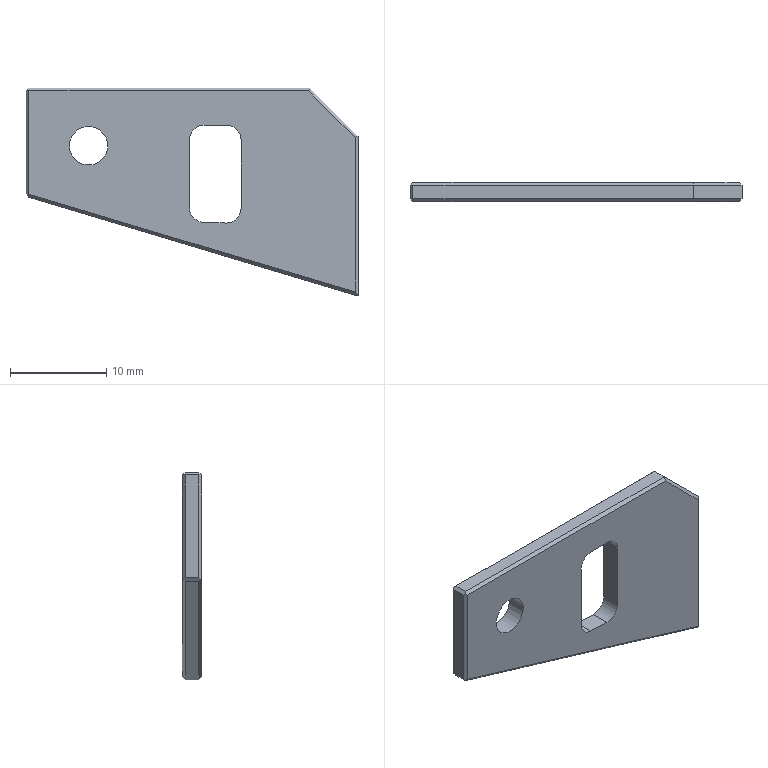Part | NX | 1 solid | 29 faces | box 34.5 x 2 x 21.6 mm | volume 969.552 mm3 | plane 23 | cylinder 6 | commonest cylinder face diameters 3 x4 4 x2
STEP:
#1=CARTESIAN_POINT('',(-158.,156.8,-47.2));
#2=VERTEX_POINT('',#1);
#3=CARTESIAN_POINT('',(-158.,158.2,-47.2));
#4=VERTEX_POINT('',#3);
#5=CARTESIAN_POINT('',(-158.,157.5,-47.2));
#6=DIRECTION('',(0.,1.,0.));
#7=VECTOR('',#6,1000.);
#8=LINE('',#5,#7);
#9=EDGE_CURVE('',#2,#4,#8,.T.);
#10=ORIENTED_EDGE('',*,*,#9,.T.);
#11=CARTESIAN_POINT('',(-158.,158.2,-57.85));
#12=VERTEX_POINT('',#11);
#13=CARTESIAN_POINT('',(-158.,158.2,-52.525));
#14=DIRECTION('',(0.,0.,1.));
#15=VECTOR('',#14,1000.);
#16=LINE('',#13,#15);
#17=EDGE_CURVE('',#12,#4,#16,.T.);
#18=ORIENTED_EDGE('',*,*,#17,.F.);
#19=CARTESIAN_POINT('',(-158.,156.8,-57.85));
#20=VERTEX_POINT('',#19);
#21=CARTESIAN_POINT('',(-158.,157.5,-57.85));
#22=DIRECTION('',(0.,1.,0.));
#23=VECTOR('',#22,1000.);
#24=LINE('',#21,#23);
#25=EDGE_CURVE('',#20,#12,#24,.T.);
#26=ORIENTED_EDGE('',*,*,#25,.F.);
#27=CARTESIAN_POINT('',(-158.,156.8,-52.525));
#28=DIRECTION('',(0.,0.,1.));
#29=VECTOR('',#28,1000.);
#30=LINE('',#27,#29);
#31=EDGE_CURVE('',#20,#2,#30,.T.);
#32=ORIENTED_EDGE('',*,*,#31,.T.);
#33=EDGE_LOOP('',(#10,#18,#26,#32));
#34=FACE_BOUND('',#33,.T.);
#35=CARTESIAN_POINT('',(-158.,156.5,-42.9));
#36=DIRECTION('',(-1.,0.,0.));
#37=DIRECTION('',(0.,0.,1.));
#38=AXIS2_PLACEMENT_3D('',#35,#36,#37);
#39=PLANE('',#38);
#40=ADVANCED_FACE('',(#34),#39,.T.);
#41=CARTESIAN_POINT('',(-128.5,156.8,-46.9));
#42=VERTEX_POINT('',#41);
#43=CARTESIAN_POINT('',(-128.5,158.2,-46.9));
#44=VERTEX_POINT('',#43);
#45=CARTESIAN_POINT('',(-128.5,157.5,-46.9));
#46=DIRECTION('',(0.,1.,0.));
#47=VECTOR('',#46,1000.);
#48=LINE('',#45,#47);
#49=EDGE_CURVE('',#42,#44,#48,.T.);
#50=ORIENTED_EDGE('',*,*,#49,.T.);
#51=CARTESIAN_POINT('',(-157.7,158.2,-46.9));
#52=VERTEX_POINT('',#51);
#53=CARTESIAN_POINT('',(-143.25,158.2,-46.9));
#54=DIRECTION('',(1.,0.,0.));
#55=VECTOR('',#54,1000.);
#56=LINE('',#53,#55);
#57=EDGE_CURVE('',#52,#44,#56,.T.);
#58=ORIENTED_EDGE('',*,*,#57,.F.);
#59=CARTESIAN_POINT('',(-157.7,156.8,-46.9));
#60=VERTEX_POINT('',#59);
#61=CARTESIAN_POINT('',(-157.7,157.5,-46.9));
#62=DIRECTION('',(0.,1.,0.));
#63=VECTOR('',#62,1000.);
#64=LINE('',#61,#63);
#65=EDGE_CURVE('',#60,#52,#64,.T.);
#66=ORIENTED_EDGE('',*,*,#65,.F.);
#67=CARTESIAN_POINT('',(-143.25,156.8,-46.9));
#68=DIRECTION('',(1.,0.,0.));
#69=VECTOR('',#68,1000.);
#70=LINE('',#67,#69);
#71=EDGE_CURVE('',#60,#42,#70,.T.);
#72=ORIENTED_EDGE('',*,*,#71,.T.);
#73=EDGE_LOOP('',(#50,#58,#66,#72));
#74=FACE_BOUND('',#73,.T.);
#75=CARTESIAN_POINT('',(-123.5,156.5,-46.9));
#76=DIRECTION('',(0.,0.,1.));
#77=DIRECTION('',(0.,-1.,0.));
#78=AXIS2_PLACEMENT_3D('',#75,#76,#77);
#79=PLANE('',#78);
#80=ADVANCED_FACE('',(#74),#79,.T.);
#81=CARTESIAN_POINT('',(-123.5,158.2,-51.9));
#82=VERTEX_POINT('',#81);
#83=CARTESIAN_POINT('',(-123.5,158.2,-68.5));
#84=VERTEX_POINT('',#83);
#85=CARTESIAN_POINT('',(-123.5,158.2,-60.2));
#86=DIRECTION('',(0.,0.,-1.));
#87=VECTOR('',#86,1000.);
#88=LINE('',#85,#87);
#89=EDGE_CURVE('',#82,#84,#88,.T.);
#90=ORIENTED_EDGE('',*,*,#89,.F.);
#91=CARTESIAN_POINT('',(-123.5,156.8,-51.9));
#92=VERTEX_POINT('',#91);
#93=CARTESIAN_POINT('',(-123.5,157.5,-51.9));
#94=DIRECTION('',(0.,1.,0.));
#95=VECTOR('',#94,1000.);
#96=LINE('',#93,#95);
#97=EDGE_CURVE('',#92,#82,#96,.T.);
#98=ORIENTED_EDGE('',*,*,#97,.F.);
#99=CARTESIAN_POINT('',(-123.5,156.8,-68.5));
#100=VERTEX_POINT('',#99);
#101=CARTESIAN_POINT('',(-123.5,156.8,-60.2));
#102=DIRECTION('',(0.,0.,-1.));
#103=VECTOR('',#102,1000.);
#104=LINE('',#101,#103);
#105=EDGE_CURVE('',#92,#100,#104,.T.);
#106=ORIENTED_EDGE('',*,*,#105,.T.);
#107=CARTESIAN_POINT('',(-123.5,156.5,-68.5));
#108=DIRECTION('',(0.,-1.,0.));
#109=VECTOR('',#108,1000.);
#110=LINE('',#107,#109);
#111=EDGE_CURVE('',#84,#100,#110,.T.);
#112=ORIENTED_EDGE('',*,*,#111,.F.);
#113=EDGE_LOOP('',(#90,#98,#106,#112));
#114=FACE_BOUND('',#113,.T.);
#115=CARTESIAN_POINT('',(-123.5,156.5,-67.9));
#116=DIRECTION('',(1.,0.,0.));
#117=DIRECTION('',(0.,1.,0.));
#118=AXIS2_PLACEMENT_3D('',#115,#116,#117);
#119=PLANE('',#118);
#120=ADVANCED_FACE('',(#114),#119,.T.);
#121=CARTESIAN_POINT('',(-135.65,156.5,-59.427));
#122=VERTEX_POINT('',#121);
#123=CARTESIAN_POINT('',(-135.65,158.5,-59.427));
#124=VERTEX_POINT('',#123);
#125=CARTESIAN_POINT('',(-135.65,156.5,-59.427));
#126=DIRECTION('',(0.,1.,0.));
#127=VECTOR('',#126,1000.);
#128=LINE('',#125,#127);
#129=EDGE_CURVE('',#122,#124,#128,.T.);
#130=ORIENTED_EDGE('',*,*,#129,.T.);
#131=CARTESIAN_POINT('',(-137.197,158.5,-60.926));
#132=VERTEX_POINT('',#131);
#133=CARTESIAN_POINT('',(-137.15,158.5,-59.427));
#134=DIRECTION('',(0.,1.,0.));
#135=DIRECTION('',(-1.,0.,0.));
#136=AXIS2_PLACEMENT_3D('',#133,#134,#135);
#137=CIRCLE('',#136,1.5);
#138=EDGE_CURVE('',#124,#132,#137,.T.);
#139=ORIENTED_EDGE('',*,*,#138,.T.);
#140=CARTESIAN_POINT('',(-137.197,156.5,-60.926));
#141=VERTEX_POINT('',#140);
#142=CARTESIAN_POINT('',(-137.197,156.5,-60.926));
#143=DIRECTION('',(0.,1.,0.));
#144=VECTOR('',#143,1000.);
#145=LINE('',#142,#144);
#146=EDGE_CURVE('',#141,#132,#145,.T.);
#147=ORIENTED_EDGE('',*,*,#146,.F.);
#148=CARTESIAN_POINT('',(-137.15,156.5,-59.427));
#149=DIRECTION('',(0.,1.,0.));
#150=DIRECTION('',(-1.,0.,0.));
#151=AXIS2_PLACEMENT_3D('',#148,#149,#150);
#152=CIRCLE('',#151,1.5);
#153=EDGE_CURVE('',#122,#141,#152,.T.);
#154=ORIENTED_EDGE('',*,*,#153,.F.);
#155=EDGE_LOOP('',(#130,#139,#147,#154));
#156=FACE_BOUND('',#155,.T.);
#157=CARTESIAN_POINT('',(-137.15,156.5,-59.427));
#158=DIRECTION('',(0.,1.,0.));
#159=DIRECTION('',(-1.,0.,0.));
#160=AXIS2_PLACEMENT_3D('',#157,#158,#159);
#161=CYLINDRICAL_SURFACE('',#160,1.5);
#162=ADVANCED_FACE('',(#156),#161,.F.);
#163=ORIENTED_EDGE('',*,*,#111,.T.);
#164=CARTESIAN_POINT('',(-157.713,156.8,-58.236));
#165=VERTEX_POINT('',#164);
#166=CARTESIAN_POINT('',(-140.75,156.8,-63.325));
#167=DIRECTION('',(-0.9578,0.,0.2873));
#168=VECTOR('',#167,1000.);
#169=LINE('',#166,#168);
#170=EDGE_CURVE('',#100,#165,#169,.T.);
#171=ORIENTED_EDGE('',*,*,#170,.T.);
#172=CARTESIAN_POINT('',(-157.713,158.2,-58.236));
#173=VERTEX_POINT('',#172);
#174=CARTESIAN_POINT('',(-157.713,157.5,-58.236));
#175=DIRECTION('',(0.,1.,0.));
#176=VECTOR('',#175,1000.);
#177=LINE('',#174,#176);
#178=EDGE_CURVE('',#165,#173,#177,.T.);
#179=ORIENTED_EDGE('',*,*,#178,.T.);
#180=CARTESIAN_POINT('',(-140.75,158.2,-63.325));
#181=DIRECTION('',(-0.9578,0.,0.2873));
#182=VECTOR('',#181,1000.);
#183=LINE('',#180,#182);
#184=EDGE_CURVE('',#84,#173,#183,.T.);
#185=ORIENTED_EDGE('',*,*,#184,.F.);
#186=EDGE_LOOP('',(#163,#171,#179,#185));
#187=FACE_BOUND('',#186,.T.);
#188=CARTESIAN_POINT('',(-160.5,156.5,-57.4));
#189=DIRECTION('',(-0.2873,0.,-0.9578));
#190=DIRECTION('',(-0.9578,0.,0.2873));
#191=AXIS2_PLACEMENT_3D('',#188,#189,#190);
#192=PLANE('',#191);
#193=ADVANCED_FACE('',(#187),#192,.T.);
#194=CARTESIAN_POINT('',(-141.001,156.5,-59.354));
#195=VERTEX_POINT('',#194);
#196=CARTESIAN_POINT('',(-141.001,158.5,-59.354));
#197=VERTEX_POINT('',#196);
#198=CARTESIAN_POINT('',(-141.001,156.5,-59.354));
#199=DIRECTION('',(0.,1.,0.));
#200=VECTOR('',#199,1000.);
#201=LINE('',#198,#200);
#202=EDGE_CURVE('',#195,#197,#201,.T.);
#203=ORIENTED_EDGE('',*,*,#202,.F.);
#204=CARTESIAN_POINT('',(-139.548,156.5,-60.853));
#205=VERTEX_POINT('',#204);
#206=CARTESIAN_POINT('',(-139.501,156.5,-59.354));
#207=DIRECTION('',(0.,1.,0.));
#208=DIRECTION('',(-1.,0.,0.));
#209=AXIS2_PLACEMENT_3D('',#206,#207,#208);
#210=CIRCLE('',#209,1.5);
#211=EDGE_CURVE('',#205,#195,#210,.T.);
#212=ORIENTED_EDGE('',*,*,#211,.F.);
#213=CARTESIAN_POINT('',(-139.548,158.5,-60.853));
#214=VERTEX_POINT('',#213);
#215=CARTESIAN_POINT('',(-139.548,156.5,-60.853));
#216=DIRECTION('',(0.,1.,0.));
#217=VECTOR('',#216,1000.);
#218=LINE('',#215,#217);
#219=EDGE_CURVE('',#205,#214,#218,.T.);
#220=ORIENTED_EDGE('',*,*,#219,.T.);
#221=CARTESIAN_POINT('',(-139.501,158.5,-59.354));
#222=DIRECTION('',(0.,1.,0.));
#223=DIRECTION('',(-1.,0.,0.));
#224=AXIS2_PLACEMENT_3D('',#221,#222,#223);
#225=CIRCLE('',#224,1.5);
#226=EDGE_CURVE('',#214,#197,#225,.T.);
#227=ORIENTED_EDGE('',*,*,#226,.T.);
#228=EDGE_LOOP('',(#203,#212,#220,#227));
#229=FACE_BOUND('',#228,.T.);
#230=CARTESIAN_POINT('',(-139.501,156.5,-59.354));
#231=DIRECTION('',(0.,1.,0.));
#232=DIRECTION('',(-1.,0.,0.));
#233=AXIS2_PLACEMENT_3D('',#230,#231,#232);
#234=CYLINDRICAL_SURFACE('',#233,1.5);
#235=ADVANCED_FACE('',(#229),#234,.F.);
#236=CARTESIAN_POINT('',(-137.15,156.5,-50.763));
#237=VERTEX_POINT('',#236);
#238=CARTESIAN_POINT('',(-137.15,158.5,-50.763));
#239=VERTEX_POINT('',#238);
#240=CARTESIAN_POINT('',(-137.15,156.5,-50.763));
#241=DIRECTION('',(0.,1.,0.));
#242=VECTOR('',#241,1000.);
#243=LINE('',#240,#242);
#244=EDGE_CURVE('',#237,#239,#243,.T.);
#245=ORIENTED_EDGE('',*,*,#244,.F.);
#246=CARTESIAN_POINT('',(-139.501,156.5,-50.763));
#247=VERTEX_POINT('',#246);
#248=CARTESIAN_POINT('',(-108.092,156.5,-50.763));
#249=DIRECTION('',(1.,0.,0.));
#250=VECTOR('',#249,1000.);
#251=LINE('',#248,#250);
#252=EDGE_CURVE('',#247,#237,#251,.T.);
#253=ORIENTED_EDGE('',*,*,#252,.F.);
#254=CARTESIAN_POINT('',(-139.501,158.5,-50.763));
#255=VERTEX_POINT('',#254);
#256=CARTESIAN_POINT('',(-139.501,156.5,-50.763));
#257=DIRECTION('',(0.,1.,0.));
#258=VECTOR('',#257,1000.);
#259=LINE('',#256,#258);
#260=EDGE_CURVE('',#247,#255,#259,.T.);
#261=ORIENTED_EDGE('',*,*,#260,.T.);
#262=CARTESIAN_POINT('',(-108.092,158.5,-50.763));
#263=DIRECTION('',(1.,0.,0.));
#264=VECTOR('',#263,1000.);
#265=LINE('',#262,#264);
#266=EDGE_CURVE('',#255,#239,#265,.T.);
#267=ORIENTED_EDGE('',*,*,#266,.T.);
#268=EDGE_LOOP('',(#245,#253,#261,#267));
#269=FACE_BOUND('',#268,.T.);
#270=CARTESIAN_POINT('',(-135.65,156.3,-50.763));
#271=DIRECTION('',(0.,0.,1.));
#272=DIRECTION('',(0.,-1.,0.));
#273=AXIS2_PLACEMENT_3D('',#270,#271,#272);
#274=PLANE('',#273);
#275=ADVANCED_FACE('',(#269),#274,.F.);
#276=ORIENTED_EDGE('',*,*,#129,.F.);
#277=CARTESIAN_POINT('',(-135.65,156.5,-52.263));
#278=VERTEX_POINT('',#277);
#279=CARTESIAN_POINT('',(-135.65,156.5,-58.685));
#280=DIRECTION('',(0.,0.,-1.));
#281=VECTOR('',#280,1000.);
#282=LINE('',#279,#281);
#283=EDGE_CURVE('',#278,#122,#282,.T.);
#284=ORIENTED_EDGE('',*,*,#283,.F.);
#285=CARTESIAN_POINT('',(-135.65,158.5,-52.263));
#286=VERTEX_POINT('',#285);
#287=CARTESIAN_POINT('',(-135.65,156.5,-52.263));
#288=DIRECTION('',(0.,1.,0.));
#289=VECTOR('',#288,1000.);
#290=LINE('',#287,#289);
#291=EDGE_CURVE('',#278,#286,#290,.T.);
#292=ORIENTED_EDGE('',*,*,#291,.T.);
#293=CARTESIAN_POINT('',(-135.65,158.5,-58.685));
#294=DIRECTION('',(0.,0.,-1.));
#295=VECTOR('',#294,1000.);
#296=LINE('',#293,#295);
#297=EDGE_CURVE('',#286,#124,#296,.T.);
#298=ORIENTED_EDGE('',*,*,#297,.T.);
#299=EDGE_LOOP('',(#276,#284,#292,#298));
#300=FACE_BOUND('',#299,.T.);
#301=CARTESIAN_POINT('',(-135.65,156.3,-60.975));
#302=DIRECTION('',(1.,0.,0.));
#303=DIRECTION('',(0.,0.,-1.));
#304=AXIS2_PLACEMENT_3D('',#301,#302,#303);
#305=PLANE('',#304);
#306=ADVANCED_FACE('',(#300),#305,.F.);
#307=CARTESIAN_POINT('',(-108.092,158.5,-61.836));
#308=DIRECTION('',(-0.9995,0.,0.03124));
#309=VECTOR('',#308,1000.);
#310=LINE('',#307,#309);
#311=EDGE_CURVE('',#132,#214,#310,.T.);
#312=ORIENTED_EDGE('',*,*,#311,.T.);
#313=ORIENTED_EDGE('',*,*,#219,.F.);
#314=CARTESIAN_POINT('',(-108.092,156.5,-61.836));
#315=DIRECTION('',(-0.9995,0.,0.03124));
#316=VECTOR('',#315,1000.);
#317=LINE('',#314,#316);
#318=EDGE_CURVE('',#141,#205,#317,.T.);
#319=ORIENTED_EDGE('',*,*,#318,.F.);
#320=ORIENTED_EDGE('',*,*,#146,.T.);
#321=EDGE_LOOP('',(#312,#313,#319,#320));
#322=FACE_BOUND('',#321,.T.);
#323=CARTESIAN_POINT('',(-141.001,156.3,-60.807));
#324=DIRECTION('',(-0.03124,0.,-0.9995));
#325=DIRECTION('',(-0.9995,0.,0.03124));
#326=AXIS2_PLACEMENT_3D('',#323,#324,#325);
#327=PLANE('',#326);
#328=ADVANCED_FACE('',(#322),#327,.F.);
#329=ORIENTED_EDGE('',*,*,#202,.T.);
#330=CARTESIAN_POINT('',(-141.001,158.5,-52.263));
#331=VERTEX_POINT('',#330);
#332=CARTESIAN_POINT('',(-141.001,158.5,-58.685));
#333=DIRECTION('',(0.,0.,1.));
#334=VECTOR('',#333,1000.);
#335=LINE('',#332,#334);
#336=EDGE_CURVE('',#197,#331,#335,.T.);
#337=ORIENTED_EDGE('',*,*,#336,.T.);
#338=CARTESIAN_POINT('',(-141.001,156.5,-52.263));
#339=VERTEX_POINT('',#338);
#340=CARTESIAN_POINT('',(-141.001,156.5,-52.263));
#341=DIRECTION('',(0.,1.,0.));
#342=VECTOR('',#341,1000.);
#343=LINE('',#340,#342);
#344=EDGE_CURVE('',#339,#331,#343,.T.);
#345=ORIENTED_EDGE('',*,*,#344,.F.);
#346=CARTESIAN_POINT('',(-141.001,156.5,-58.685));
#347=DIRECTION('',(0.,0.,1.));
#348=VECTOR('',#347,1000.);
#349=LINE('',#346,#348);
#350=EDGE_CURVE('',#195,#339,#349,.T.);
#351=ORIENTED_EDGE('',*,*,#350,.F.);
#352=EDGE_LOOP('',(#329,#337,#345,#351));
#353=FACE_BOUND('',#352,.T.);
#354=CARTESIAN_POINT('',(-141.001,156.3,-50.763));
#355=DIRECTION('',(-1.,0.,0.));
#356=DIRECTION('',(0.,0.,1.));
#357=AXIS2_PLACEMENT_3D('',#354,#355,#356);
#358=PLANE('',#357);
#359=ADVANCED_FACE('',(#353),#358,.F.);
#360=ORIENTED_EDGE('',*,*,#344,.T.);
#361=CARTESIAN_POINT('',(-139.501,158.5,-52.263));
#362=DIRECTION('',(0.,1.,0.));
#363=DIRECTION('',(-1.,0.,0.));
#364=AXIS2_PLACEMENT_3D('',#361,#362,#363);
#365=CIRCLE('',#364,1.5);
#366=EDGE_CURVE('',#331,#255,#365,.T.);
#367=ORIENTED_EDGE('',*,*,#366,.T.);
#368=ORIENTED_EDGE('',*,*,#260,.F.);
#369=CARTESIAN_POINT('',(-139.501,156.5,-52.263));
#370=DIRECTION('',(0.,1.,0.));
#371=DIRECTION('',(-1.,0.,0.));
#372=AXIS2_PLACEMENT_3D('',#369,#370,#371);
#373=CIRCLE('',#372,1.5);
#374=EDGE_CURVE('',#339,#247,#373,.T.);
#375=ORIENTED_EDGE('',*,*,#374,.F.);
#376=EDGE_LOOP('',(#360,#367,#368,#375));
#377=FACE_BOUND('',#376,.T.);
#378=CARTESIAN_POINT('',(-139.501,156.5,-52.263));
#379=DIRECTION('',(0.,1.,0.));
#380=DIRECTION('',(-1.,0.,0.));
#381=AXIS2_PLACEMENT_3D('',#378,#379,#380);
#382=CYLINDRICAL_SURFACE('',#381,1.5);
#383=ADVANCED_FACE('',(#377),#382,.F.);
#384=ORIENTED_EDGE('',*,*,#244,.T.);
#385=CARTESIAN_POINT('',(-137.15,158.5,-52.263));
#386=DIRECTION('',(0.,1.,0.));
#387=DIRECTION('',(-1.,0.,0.));
#388=AXIS2_PLACEMENT_3D('',#385,#386,#387);
#389=CIRCLE('',#388,1.5);
#390=EDGE_CURVE('',#239,#286,#389,.T.);
#391=ORIENTED_EDGE('',*,*,#390,.T.);
#392=ORIENTED_EDGE('',*,*,#291,.F.);
#393=CARTESIAN_POINT('',(-137.15,156.5,-52.263));
#394=DIRECTION('',(0.,1.,0.));
#395=DIRECTION('',(-1.,0.,0.));
#396=AXIS2_PLACEMENT_3D('',#393,#394,#395);
#397=CIRCLE('',#396,1.5);
#398=EDGE_CURVE('',#237,#278,#397,.T.);
#399=ORIENTED_EDGE('',*,*,#398,.F.);
#400=EDGE_LOOP('',(#384,#391,#392,#399));
#401=FACE_BOUND('',#400,.T.);
#402=CARTESIAN_POINT('',(-137.15,156.5,-52.263));
#403=DIRECTION('',(0.,1.,0.));
#404=DIRECTION('',(-1.,0.,0.));
#405=AXIS2_PLACEMENT_3D('',#402,#403,#404);
#406=CYLINDRICAL_SURFACE('',#405,1.5);
#407=ADVANCED_FACE('',(#401),#406,.F.);
#408=CARTESIAN_POINT('',(-126.,158.2,-49.4));
#409=DIRECTION('',(-0.7071,0.,0.7071));
#410=VECTOR('',#409,1000.);
#411=LINE('',#408,#410);
#412=EDGE_CURVE('',#82,#44,#411,.T.);
#413=ORIENTED_EDGE('',*,*,#412,.T.);
#414=ORIENTED_EDGE('',*,*,#49,.F.);
#415=CARTESIAN_POINT('',(-126.,156.8,-49.4));
#416=DIRECTION('',(-0.7071,0.,0.7071));
#417=VECTOR('',#416,1000.);
#418=LINE('',#415,#417);
#419=EDGE_CURVE('',#92,#42,#418,.T.);
#420=ORIENTED_EDGE('',*,*,#419,.F.);
#421=ORIENTED_EDGE('',*,*,#97,.T.);
#422=EDGE_LOOP('',(#413,#414,#420,#421));
#423=FACE_BOUND('',#422,.T.);
#424=CARTESIAN_POINT('',(-126.,157.5,-49.4));
#425=DIRECTION('',(0.7071,0.,0.7071));
#426=DIRECTION('',(0.,-1.,0.));
#427=AXIS2_PLACEMENT_3D('',#424,#425,#426);
#428=PLANE('',#427);
#429=ADVANCED_FACE('',(#423),#428,.T.);
#430=ORIENTED_EDGE('',*,*,#25,.T.);
#431=CARTESIAN_POINT('',(-157.856,158.344,-58.043));
#432=VERTEX_POINT('',#431);
#433=CARTESIAN_POINT('',(-157.379,158.821,-58.685));
#434=DIRECTION('',(0.5126,0.5126,-0.6889));
#435=VECTOR('',#434,1000.);
#436=LINE('',#433,#435);
#437=EDGE_CURVE('',#12,#432,#436,.T.);
#438=ORIENTED_EDGE('',*,*,#437,.T.);
#439=CARTESIAN_POINT('',(-157.379,157.866,-58.685));
#440=DIRECTION('',(0.5126,-0.5126,-0.6889));
#441=VECTOR('',#440,1000.);
#442=LINE('',#439,#441);
#443=EDGE_CURVE('',#432,#173,#442,.T.);
#444=ORIENTED_EDGE('',*,*,#443,.T.);
#445=ORIENTED_EDGE('',*,*,#178,.F.);
#446=CARTESIAN_POINT('',(-157.856,156.656,-58.043));
#447=VERTEX_POINT('',#446);
#448=CARTESIAN_POINT('',(-157.379,157.134,-58.685));
#449=DIRECTION('',(0.5126,0.5126,-0.6889));
#450=VECTOR('',#449,1000.);
#451=LINE('',#448,#450);
#452=EDGE_CURVE('',#447,#165,#451,.T.);
#453=ORIENTED_EDGE('',*,*,#452,.F.);
#454=CARTESIAN_POINT('',(-157.379,156.179,-58.685));
#455=DIRECTION('',(0.5126,-0.5126,-0.6889));
#456=VECTOR('',#455,1000.);
#457=LINE('',#454,#456);
#458=EDGE_CURVE('',#20,#447,#457,.T.);
#459=ORIENTED_EDGE('',*,*,#458,.F.);
#460=EDGE_LOOP('',(#430,#438,#444,#445,#453,#459));
#461=FACE_BOUND('',#460,.T.);
#462=CARTESIAN_POINT('',(-157.856,157.5,-58.043));
#463=DIRECTION('',(0.8023,0.,0.5969));
#464=DIRECTION('',(0.,-1.,0.));
#465=AXIS2_PLACEMENT_3D('',#462,#463,#464);
#466=PLANE('',#465);
#467=ADVANCED_FACE('',(#461),#466,.F.);
#468=ORIENTED_EDGE('',*,*,#9,.F.);
#469=CARTESIAN_POINT('',(-157.85,156.65,-47.05));
#470=VERTEX_POINT('',#469);
#471=CARTESIAN_POINT('',(-169.485,168.285,-58.685));
#472=DIRECTION('',(0.5774,-0.5774,0.5774));
#473=VECTOR('',#472,1000.);
#474=LINE('',#471,#473);
#475=EDGE_CURVE('',#2,#470,#474,.T.);
#476=ORIENTED_EDGE('',*,*,#475,.T.);
#477=CARTESIAN_POINT('',(-169.485,145.015,-58.685));
#478=DIRECTION('',(0.5774,0.5774,0.5774));
#479=VECTOR('',#478,1000.);
#480=LINE('',#477,#479);
#481=EDGE_CURVE('',#470,#60,#480,.T.);
#482=ORIENTED_EDGE('',*,*,#481,.T.);
#483=ORIENTED_EDGE('',*,*,#65,.T.);
#484=CARTESIAN_POINT('',(-157.85,158.35,-47.05));
#485=VERTEX_POINT('',#484);
#486=CARTESIAN_POINT('',(-169.485,169.985,-58.685));
#487=DIRECTION('',(0.5774,-0.5774,0.5774));
#488=VECTOR('',#487,1000.);
#489=LINE('',#486,#488);
#490=EDGE_CURVE('',#485,#52,#489,.T.);
#491=ORIENTED_EDGE('',*,*,#490,.F.);
#492=CARTESIAN_POINT('',(-169.485,146.715,-58.685));
#493=DIRECTION('',(0.5774,0.5774,0.5774));
#494=VECTOR('',#493,1000.);
#495=LINE('',#492,#494);
#496=EDGE_CURVE('',#4,#485,#495,.T.);
#497=ORIENTED_EDGE('',*,*,#496,.F.);
#498=EDGE_LOOP('',(#468,#476,#482,#483,#491,#497));
#499=FACE_BOUND('',#498,.T.);
#500=CARTESIAN_POINT('',(-157.85,157.5,-47.05));
#501=DIRECTION('',(-0.7071,0.,0.7071));
#502=DIRECTION('',(0.,1.,0.));
#503=AXIS2_PLACEMENT_3D('',#500,#501,#502);
#504=PLANE('',#503);
#505=ADVANCED_FACE('',(#499),#504,.T.);
#506=ORIENTED_EDGE('',*,*,#419,.T.);
#507=CARTESIAN_POINT('',(-128.624,156.5,-47.2));
#508=VERTEX_POINT('',#507);
#509=CARTESIAN_POINT('',(-133.381,145.015,-58.685));
#510=DIRECTION('',(0.2811,0.6786,0.6786));
#511=VECTOR('',#510,1000.);
#512=LINE('',#509,#511);
#513=EDGE_CURVE('',#508,#42,#512,.T.);
#514=ORIENTED_EDGE('',*,*,#513,.F.);
#515=CARTESIAN_POINT('',(-123.8,156.5,-52.024));
#516=VERTEX_POINT('',#515);
#517=CARTESIAN_POINT('',(-126.212,156.5,-49.612));
#518=DIRECTION('',(-0.7071,0.,0.7071));
#519=VECTOR('',#518,1000.);
#520=LINE('',#517,#519);
#521=EDGE_CURVE('',#516,#508,#520,.T.);
#522=ORIENTED_EDGE('',*,*,#521,.F.);
#523=CARTESIAN_POINT('',(-108.092,172.208,-45.518));
#524=DIRECTION('',(-0.6786,-0.6786,-0.2811));
#525=VECTOR('',#524,1000.);
#526=LINE('',#523,#525);
#527=EDGE_CURVE('',#92,#516,#526,.T.);
#528=ORIENTED_EDGE('',*,*,#527,.F.);
#529=EDGE_LOOP('',(#506,#514,#522,#528));
#530=FACE_BOUND('',#529,.T.);
#531=CARTESIAN_POINT('',(-126.106,156.65,-49.506));
#532=DIRECTION('',(-0.5,0.7071,-0.5));
#533=DIRECTION('',(-0.7071,0.,0.7071));
#534=AXIS2_PLACEMENT_3D('',#531,#532,#533);
#535=PLANE('',#534);
#536=ADVANCED_FACE('',(#530),#535,.F.);
#537=ORIENTED_EDGE('',*,*,#412,.F.);
#538=CARTESIAN_POINT('',(-123.8,158.5,-52.024));
#539=VERTEX_POINT('',#538);
#540=CARTESIAN_POINT('',(-108.092,142.792,-45.518));
#541=DIRECTION('',(0.6786,-0.6786,0.2811));
#542=VECTOR('',#541,1000.);
#543=LINE('',#540,#542);
#544=EDGE_CURVE('',#539,#82,#543,.T.);
#545=ORIENTED_EDGE('',*,*,#544,.F.);
#546=CARTESIAN_POINT('',(-128.624,158.5,-47.2));
#547=VERTEX_POINT('',#546);
#548=CARTESIAN_POINT('',(-126.212,158.5,-49.612));
#549=DIRECTION('',(-0.7071,0.,0.7071));
#550=VECTOR('',#549,1000.);
#551=LINE('',#548,#550);
#552=EDGE_CURVE('',#539,#547,#551,.T.);
#553=ORIENTED_EDGE('',*,*,#552,.T.);
#554=CARTESIAN_POINT('',(-133.381,169.985,-58.685));
#555=DIRECTION('',(-0.2811,0.6786,-0.6786));
#556=VECTOR('',#555,1000.);
#557=LINE('',#554,#556);
#558=EDGE_CURVE('',#44,#547,#557,.T.);
#559=ORIENTED_EDGE('',*,*,#558,.F.);
#560=EDGE_LOOP('',(#537,#545,#553,#559));
#561=FACE_BOUND('',#560,.T.);
#562=CARTESIAN_POINT('',(-126.106,158.35,-49.506));
#563=DIRECTION('',(0.5,0.7071,0.5));
#564=DIRECTION('',(0.7071,0.,-0.7071));
#565=AXIS2_PLACEMENT_3D('',#562,#563,#564);
#566=PLANE('',#565);
#567=ADVANCED_FACE('',(#561),#566,.T.);
#568=CARTESIAN_POINT('',(-149.5,158.5,-52.9));
#569=VERTEX_POINT('',#568);
#570=CARTESIAN_POINT('',(-153.5,158.5,-52.9));
#571=VERTEX_POINT('',#570);
#572=CARTESIAN_POINT('',(-151.5,158.5,-52.9));
#573=DIRECTION('',(0.,1.,0.));
#574=DIRECTION('',(-1.,0.,0.));
#575=AXIS2_PLACEMENT_3D('',#572,#573,#574);
#576=CIRCLE('',#575,2.);
#577=EDGE_CURVE('',#569,#571,#576,.T.);
#578=ORIENTED_EDGE('',*,*,#577,.T.);
#579=CARTESIAN_POINT('',(-153.5,156.5,-52.9));
#580=VERTEX_POINT('',#579);
#581=CARTESIAN_POINT('',(-153.5,156.5,-52.9));
#582=DIRECTION('',(0.,1.,0.));
#583=VECTOR('',#582,1000.);
#584=LINE('',#581,#583);
#585=EDGE_CURVE('',#571,#580,#584,.F.);
#586=ORIENTED_EDGE('',*,*,#585,.T.);
#587=CARTESIAN_POINT('',(-149.5,156.5,-52.9));
#588=VERTEX_POINT('',#587);
#589=CARTESIAN_POINT('',(-151.5,156.5,-52.9));
#590=DIRECTION('',(0.,1.,0.));
#591=DIRECTION('',(-1.,0.,0.));
#592=AXIS2_PLACEMENT_3D('',#589,#590,#591);
#593=CIRCLE('',#592,2.);
#594=EDGE_CURVE('',#588,#580,#593,.T.);
#595=ORIENTED_EDGE('',*,*,#594,.F.);
#596=CARTESIAN_POINT('',(-149.5,156.5,-52.9));
#597=DIRECTION('',(0.,1.,0.));
#598=VECTOR('',#597,1000.);
#599=LINE('',#596,#598);
#600=EDGE_CURVE('',#569,#588,#599,.F.);
#601=ORIENTED_EDGE('',*,*,#600,.F.);
#602=EDGE_LOOP('',(#578,#586,#595,#601));
#603=FACE_BOUND('',#602,.T.);
#604=CARTESIAN_POINT('',(-151.5,156.5,-52.9));
#605=DIRECTION('',(0.,1.,0.));
#606=DIRECTION('',(-1.,0.,0.));
#607=AXIS2_PLACEMENT_3D('',#604,#605,#606);
#608=CYLINDRICAL_SURFACE('',#607,2.);
#609=ADVANCED_FACE('',(#603),#608,.F.);
#610=ORIENTED_EDGE('',*,*,#585,.F.);
#611=CARTESIAN_POINT('',(-151.5,158.5,-52.9));
#612=DIRECTION('',(0.,1.,0.));
#613=DIRECTION('',(-1.,0.,0.));
#614=AXIS2_PLACEMENT_3D('',#611,#612,#613);
#615=CIRCLE('',#614,2.);
#616=EDGE_CURVE('',#571,#569,#615,.T.);
#617=ORIENTED_EDGE('',*,*,#616,.T.);
#618=ORIENTED_EDGE('',*,*,#600,.T.);
#619=CARTESIAN_POINT('',(-151.5,156.5,-52.9));
#620=DIRECTION('',(0.,1.,0.));
#621=DIRECTION('',(-1.,0.,0.));
#622=AXIS2_PLACEMENT_3D('',#619,#620,#621);
#623=CIRCLE('',#622,2.);
#624=EDGE_CURVE('',#580,#588,#623,.T.);
#625=ORIENTED_EDGE('',*,*,#624,.F.);
#626=EDGE_LOOP('',(#610,#617,#618,#625));
#627=FACE_BOUND('',#626,.T.);
#628=CARTESIAN_POINT('',(-151.5,156.5,-52.9));
#629=DIRECTION('',(0.,1.,0.));
#630=DIRECTION('',(-1.,0.,0.));
#631=AXIS2_PLACEMENT_3D('',#628,#629,#630);
#632=CYLINDRICAL_SURFACE('',#631,2.);
#633=ADVANCED_FACE('',(#627),#632,.F.);
#634=CARTESIAN_POINT('',(-157.7,158.5,-57.927));
#635=VERTEX_POINT('',#634);
#636=CARTESIAN_POINT('',(-157.7,158.5,-47.2));
#637=VERTEX_POINT('',#636);
#638=CARTESIAN_POINT('',(-157.7,158.5,-52.525));
#639=DIRECTION('',(0.,0.,1.));
#640=VECTOR('',#639,1000.);
#641=LINE('',#638,#640);
#642=EDGE_CURVE('',#635,#637,#641,.T.);
#643=ORIENTED_EDGE('',*,*,#642,.T.);
#644=CARTESIAN_POINT('',(-143.25,158.5,-47.2));
#645=DIRECTION('',(1.,0.,0.));
#646=VECTOR('',#645,1000.);
#647=LINE('',#644,#646);
#648=EDGE_CURVE('',#637,#547,#647,.T.);
#649=ORIENTED_EDGE('',*,*,#648,.T.);
#650=ORIENTED_EDGE('',*,*,#552,.F.);
#651=CARTESIAN_POINT('',(-123.8,158.5,-68.097));
#652=VERTEX_POINT('',#651);
#653=CARTESIAN_POINT('',(-123.8,158.5,-60.2));
#654=DIRECTION('',(0.,0.,-1.));
#655=VECTOR('',#654,1000.);
#656=LINE('',#653,#655);
#657=EDGE_CURVE('',#539,#652,#656,.T.);
#658=ORIENTED_EDGE('',*,*,#657,.T.);
#659=CARTESIAN_POINT('',(-140.664,158.5,-63.038));
#660=DIRECTION('',(-0.9578,0.,0.2873));
#661=VECTOR('',#660,1000.);
#662=LINE('',#659,#661);
#663=EDGE_CURVE('',#652,#635,#662,.T.);
#664=ORIENTED_EDGE('',*,*,#663,.T.);
#665=EDGE_LOOP('',(#643,#649,#650,#658,#664));
#666=FACE_BOUND('',#665,.T.);
#667=ORIENTED_EDGE('',*,*,#336,.F.);
#668=ORIENTED_EDGE('',*,*,#226,.F.);
#669=ORIENTED_EDGE('',*,*,#311,.F.);
#670=ORIENTED_EDGE('',*,*,#138,.F.);
#671=ORIENTED_EDGE('',*,*,#297,.F.);
#672=ORIENTED_EDGE('',*,*,#390,.F.);
#673=ORIENTED_EDGE('',*,*,#266,.F.);
#674=ORIENTED_EDGE('',*,*,#366,.F.);
#675=EDGE_LOOP('',(#667,#668,#669,#670,#671,#672,#673,#674));
#676=FACE_BOUND('',#675,.T.);
#677=ORIENTED_EDGE('',*,*,#577,.F.);
#678=ORIENTED_EDGE('',*,*,#616,.F.);
#679=EDGE_LOOP('',(#677,#678));
#680=FACE_BOUND('',#679,.T.);
#681=CARTESIAN_POINT('',(-108.092,158.5,-58.685));
#682=DIRECTION('',(0.,1.,0.));
#683=DIRECTION('',(0.,0.,-1.));
#684=AXIS2_PLACEMENT_3D('',#681,#682,#683);
#685=PLANE('',#684);
#686=ADVANCED_FACE('',(#666,#676,#680),#685,.T.);
#687=ORIENTED_EDGE('',*,*,#657,.F.);
#688=ORIENTED_EDGE('',*,*,#544,.T.);
#689=ORIENTED_EDGE('',*,*,#89,.T.);
#690=CARTESIAN_POINT('',(-130.803,165.503,-58.685));
#691=DIRECTION('',(-0.5126,0.5126,0.6889));
#692=VECTOR('',#691,1000.);
#693=LINE('',#690,#692);
#694=EDGE_CURVE('',#84,#652,#693,.T.);
#695=ORIENTED_EDGE('',*,*,#694,.T.);
#696=EDGE_LOOP('',(#687,#688,#689,#695));
#697=FACE_BOUND('',#696,.T.);
#698=CARTESIAN_POINT('',(-123.65,158.35,-60.2));
#699=DIRECTION('',(0.7071,0.7071,0.));
#700=DIRECTION('',(0.,0.,-1.));
#701=AXIS2_PLACEMENT_3D('',#698,#699,#700);
#702=PLANE('',#701);
#703=ADVANCED_FACE('',(#697),#702,.T.);
#704=ORIENTED_EDGE('',*,*,#648,.F.);
#705=CARTESIAN_POINT('',(-146.215,169.985,-58.685));
#706=DIRECTION('',(-0.5774,-0.5774,0.5774));
#707=VECTOR('',#706,1000.);
#708=LINE('',#705,#707);
#709=EDGE_CURVE('',#637,#485,#708,.T.);
#710=ORIENTED_EDGE('',*,*,#709,.T.);
#711=ORIENTED_EDGE('',*,*,#490,.T.);
#712=ORIENTED_EDGE('',*,*,#57,.T.);
#713=ORIENTED_EDGE('',*,*,#558,.T.);
#714=EDGE_LOOP('',(#704,#710,#711,#712,#713));
#715=FACE_BOUND('',#714,.T.);
#716=CARTESIAN_POINT('',(-143.25,158.35,-47.05));
#717=DIRECTION('',(0.,0.7071,0.7071));
#718=DIRECTION('',(1.,0.,0.));
#719=AXIS2_PLACEMENT_3D('',#716,#717,#718);
#720=PLANE('',#719);
#721=ADVANCED_FACE('',(#715),#720,.T.);
#722=ORIENTED_EDGE('',*,*,#663,.F.);
#723=ORIENTED_EDGE('',*,*,#694,.F.);
#724=ORIENTED_EDGE('',*,*,#184,.T.);
#725=ORIENTED_EDGE('',*,*,#443,.F.);
#726=CARTESIAN_POINT('',(-159.7,156.5,-59.415));
#727=DIRECTION('',(0.6258,0.6258,0.4656));
#728=VECTOR('',#727,1000.);
#729=LINE('',#726,#728);
#730=EDGE_CURVE('',#432,#635,#729,.T.);
#731=ORIENTED_EDGE('',*,*,#730,.T.);
#732=EDGE_LOOP('',(#722,#723,#724,#725,#731));
#733=FACE_BOUND('',#732,.T.);
#734=CARTESIAN_POINT('',(-140.707,158.35,-63.181));
#735=DIRECTION('',(-0.2032,0.7071,-0.6773));
#736=DIRECTION('',(-0.9578,0.,0.2873));
#737=AXIS2_PLACEMENT_3D('',#734,#735,#736);
#738=PLANE('',#737);
#739=ADVANCED_FACE('',(#733),#738,.T.);
#740=ORIENTED_EDGE('',*,*,#642,.F.);
#741=ORIENTED_EDGE('',*,*,#730,.F.);
#742=ORIENTED_EDGE('',*,*,#437,.F.);
#743=ORIENTED_EDGE('',*,*,#17,.T.);
#744=ORIENTED_EDGE('',*,*,#496,.T.);
#745=ORIENTED_EDGE('',*,*,#709,.F.);
#746=EDGE_LOOP('',(#740,#741,#742,#743,#744,#745));
#747=FACE_BOUND('',#746,.T.);
#748=CARTESIAN_POINT('',(-157.85,158.35,-52.525));
#749=DIRECTION('',(-0.7071,0.7071,0.));
#750=DIRECTION('',(0.,0.,1.));
#751=AXIS2_PLACEMENT_3D('',#748,#749,#750);
#752=PLANE('',#751);
#753=ADVANCED_FACE('',(#747),#752,.T.);
#754=CARTESIAN_POINT('',(-123.8,156.5,-68.097));
#755=VERTEX_POINT('',#754);
#756=CARTESIAN_POINT('',(-157.7,156.5,-57.927));
#757=VERTEX_POINT('',#756);
#758=CARTESIAN_POINT('',(-140.664,156.5,-63.038));
#759=DIRECTION('',(-0.9578,0.,0.2873));
#760=VECTOR('',#759,1000.);
#761=LINE('',#758,#760);
#762=EDGE_CURVE('',#755,#757,#761,.T.);
#763=ORIENTED_EDGE('',*,*,#762,.F.);
#764=CARTESIAN_POINT('',(-123.8,156.5,-60.2));
#765=DIRECTION('',(0.,0.,-1.));
#766=VECTOR('',#765,1000.);
#767=LINE('',#764,#766);
#768=EDGE_CURVE('',#516,#755,#767,.T.);
#769=ORIENTED_EDGE('',*,*,#768,.F.);
#770=ORIENTED_EDGE('',*,*,#521,.T.);
#771=CARTESIAN_POINT('',(-157.7,156.5,-47.2));
#772=VERTEX_POINT('',#771);
#773=CARTESIAN_POINT('',(-143.25,156.5,-47.2));
#774=DIRECTION('',(1.,0.,0.));
#775=VECTOR('',#774,1000.);
#776=LINE('',#773,#775);
#777=EDGE_CURVE('',#772,#508,#776,.T.);
#778=ORIENTED_EDGE('',*,*,#777,.F.);
#779=CARTESIAN_POINT('',(-157.7,156.5,-52.525));
#780=DIRECTION('',(0.,0.,1.));
#781=VECTOR('',#780,1000.);
#782=LINE('',#779,#781);
#783=EDGE_CURVE('',#757,#772,#782,.T.);
#784=ORIENTED_EDGE('',*,*,#783,.F.);
#785=EDGE_LOOP('',(#763,#769,#770,#778,#784));
#786=FACE_BOUND('',#785,.T.);
#787=ORIENTED_EDGE('',*,*,#350,.T.);
#788=ORIENTED_EDGE('',*,*,#374,.T.);
#789=ORIENTED_EDGE('',*,*,#252,.T.);
#790=ORIENTED_EDGE('',*,*,#398,.T.);
#791=ORIENTED_EDGE('',*,*,#283,.T.);
#792=ORIENTED_EDGE('',*,*,#153,.T.);
#793=ORIENTED_EDGE('',*,*,#318,.T.);
#794=ORIENTED_EDGE('',*,*,#211,.T.);
#795=EDGE_LOOP('',(#787,#788,#789,#790,#791,#792,#793,#794));
#796=FACE_BOUND('',#795,.T.);
#797=ORIENTED_EDGE('',*,*,#594,.T.);
#798=ORIENTED_EDGE('',*,*,#624,.T.);
#799=EDGE_LOOP('',(#797,#798));
#800=FACE_BOUND('',#799,.T.);
#801=CARTESIAN_POINT('',(-108.092,156.5,-58.685));
#802=DIRECTION('',(0.,1.,0.));
#803=DIRECTION('',(0.,0.,-1.));
#804=AXIS2_PLACEMENT_3D('',#801,#802,#803);
#805=PLANE('',#804);
#806=ADVANCED_FACE('',(#786,#796,#800),#805,.F.);
#807=ORIENTED_EDGE('',*,*,#768,.T.);
#808=CARTESIAN_POINT('',(-130.803,149.497,-58.685));
#809=DIRECTION('',(0.5126,0.5126,-0.6889));
#810=VECTOR('',#809,1000.);
#811=LINE('',#808,#810);
#812=EDGE_CURVE('',#755,#100,#811,.T.);
#813=ORIENTED_EDGE('',*,*,#812,.T.);
#814=ORIENTED_EDGE('',*,*,#105,.F.);
#815=ORIENTED_EDGE('',*,*,#527,.T.);
#816=EDGE_LOOP('',(#807,#813,#814,#815));
#817=FACE_BOUND('',#816,.T.);
#818=CARTESIAN_POINT('',(-123.65,156.65,-60.2));
#819=DIRECTION('',(-0.7071,0.7071,0.));
#820=DIRECTION('',(0.,0.,1.));
#821=AXIS2_PLACEMENT_3D('',#818,#819,#820);
#822=PLANE('',#821);
#823=ADVANCED_FACE('',(#817),#822,.F.);
#824=ORIENTED_EDGE('',*,*,#777,.T.);
#825=ORIENTED_EDGE('',*,*,#513,.T.);
#826=ORIENTED_EDGE('',*,*,#71,.F.);
#827=ORIENTED_EDGE('',*,*,#481,.F.);
#828=CARTESIAN_POINT('',(-146.215,145.015,-58.685));
#829=DIRECTION('',(0.5774,-0.5774,-0.5774));
#830=VECTOR('',#829,1000.);
#831=LINE('',#828,#830);
#832=EDGE_CURVE('',#470,#772,#831,.T.);
#833=ORIENTED_EDGE('',*,*,#832,.T.);
#834=EDGE_LOOP('',(#824,#825,#826,#827,#833));
#835=FACE_BOUND('',#834,.T.);
#836=CARTESIAN_POINT('',(-143.25,156.65,-47.05));
#837=DIRECTION('',(0.,0.7071,-0.7071));
#838=DIRECTION('',(-1.,0.,0.));
#839=AXIS2_PLACEMENT_3D('',#836,#837,#838);
#840=PLANE('',#839);
#841=ADVANCED_FACE('',(#835),#840,.F.);
#842=ORIENTED_EDGE('',*,*,#783,.T.);
#843=ORIENTED_EDGE('',*,*,#832,.F.);
#844=ORIENTED_EDGE('',*,*,#475,.F.);
#845=ORIENTED_EDGE('',*,*,#31,.F.);
#846=ORIENTED_EDGE('',*,*,#458,.T.);
#847=CARTESIAN_POINT('',(-157.7,156.5,-57.927));
#848=DIRECTION('',(0.6258,-0.6258,0.4656));
#849=VECTOR('',#848,1000.);
#850=LINE('',#847,#849);
#851=EDGE_CURVE('',#447,#757,#850,.T.);
#852=ORIENTED_EDGE('',*,*,#851,.T.);
#853=EDGE_LOOP('',(#842,#843,#844,#845,#846,#852));
#854=FACE_BOUND('',#853,.T.);
#855=CARTESIAN_POINT('',(-157.85,156.65,-52.525));
#856=DIRECTION('',(0.7071,0.7071,0.));
#857=DIRECTION('',(0.,0.,-1.));
#858=AXIS2_PLACEMENT_3D('',#855,#856,#857);
#859=PLANE('',#858);
#860=ADVANCED_FACE('',(#854),#859,.F.);
#861=ORIENTED_EDGE('',*,*,#762,.T.);
#862=ORIENTED_EDGE('',*,*,#851,.F.);
#863=ORIENTED_EDGE('',*,*,#452,.T.);
#864=ORIENTED_EDGE('',*,*,#170,.F.);
#865=ORIENTED_EDGE('',*,*,#812,.F.);
#866=EDGE_LOOP('',(#861,#862,#863,#864,#865));
#867=FACE_BOUND('',#866,.T.);
#868=CARTESIAN_POINT('',(-140.707,156.65,-63.181));
#869=DIRECTION('',(0.2032,0.7071,0.6773));
#870=DIRECTION('',(0.9578,0.,-0.2873));
#871=AXIS2_PLACEMENT_3D('',#868,#869,#870);
#872=PLANE('',#871);
#873=ADVANCED_FACE('',(#867),#872,.F.);
#874=CLOSED_SHELL('',(#40,#80,#120,#162,#193,#235,#275,#306,#328,#359,#383,#407,#429,#467,#505,#536,#567,#609,#633,#686,#703,#721,#739,#753,#806,#823,#841,#860,#873));
#875=MANIFOLD_SOLID_BREP('',#874);
#876=(LENGTH_UNIT()NAMED_UNIT(*)SI_UNIT(.MILLI.,.METRE.));
#877=UNCERTAINTY_MEASURE_WITH_UNIT(LENGTH_MEASURE(0.00001),#876,'','');
#878=(NAMED_UNIT(*)PLANE_ANGLE_UNIT()SI_UNIT($,.RADIAN.));
#879=(NAMED_UNIT(*)SI_UNIT($,.STERADIAN.)SOLID_ANGLE_UNIT());
#880=(GEOMETRIC_REPRESENTATION_CONTEXT(3)GLOBAL_UNCERTAINTY_ASSIGNED_CONTEXT((#877))GLOBAL_UNIT_ASSIGNED_CONTEXT((#876,#878,#879))REPRESENTATION_CONTEXT('',''));
#881=ADVANCED_BREP_SHAPE_REPRESENTATION('',(#875),#880);